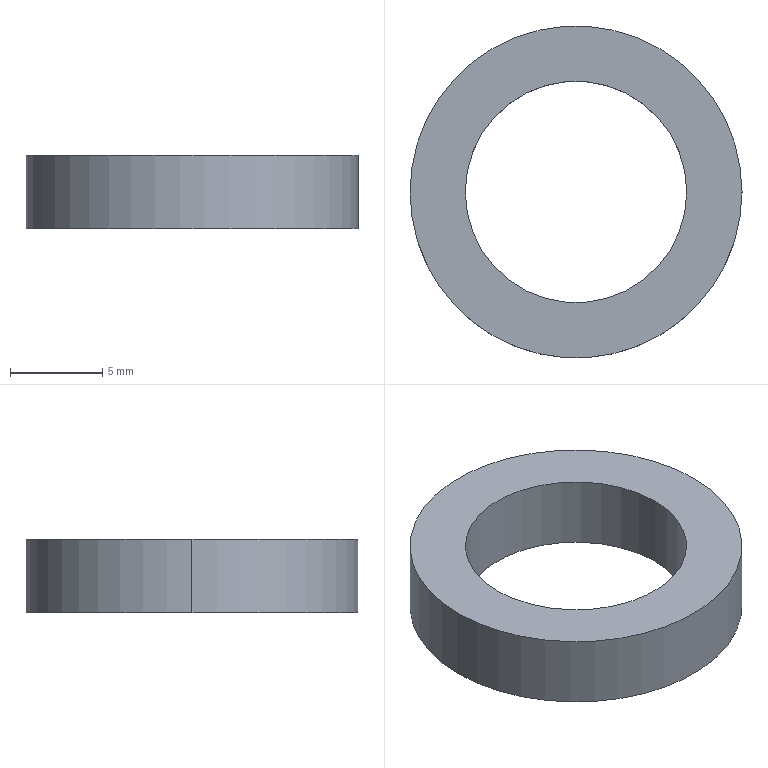Part | STEP file | 6701ZZ | 1 solid | 6 faces | box 18 x 18 x 4 mm | volume 565.487 mm3 | cylinder 4 | plane 2 | commonest cylinder face diameters 12 x2 18 x2
STEP:
#1=CARTESIAN_POINT('',(-6.,0.,4.));
#2=VERTEX_POINT('',#1);
#3=CARTESIAN_POINT('',(6.,0.,4.));
#4=VERTEX_POINT('',#3);
#5=CARTESIAN_POINT('',(0.,0.,4.));
#6=DIRECTION('',(0.,0.,1.));
#7=DIRECTION('',(1.,0.,0.));
#8=AXIS2_PLACEMENT_3D('',#5,#6,#7);
#9=CIRCLE('',#8,6.);
#10=EDGE_CURVE('',#2,#4,#9,.T.);
#11=ORIENTED_EDGE('',*,*,#10,.T.);
#12=CARTESIAN_POINT('',(6.,0.,0.));
#13=VERTEX_POINT('',#12);
#14=CARTESIAN_POINT('',(6.,0.,4.));
#15=DIRECTION('',(0.,0.,-1.));
#16=VECTOR('',#15,1000.);
#17=LINE('',#14,#16);
#18=EDGE_CURVE('',#4,#13,#17,.T.);
#19=ORIENTED_EDGE('',*,*,#18,.T.);
#20=CARTESIAN_POINT('',(-6.,0.,0.));
#21=VERTEX_POINT('',#20);
#22=CARTESIAN_POINT('',(0.,0.,0.));
#23=DIRECTION('',(0.,0.,1.));
#24=DIRECTION('',(1.,0.,0.));
#25=AXIS2_PLACEMENT_3D('',#22,#23,#24);
#26=CIRCLE('',#25,6.);
#27=EDGE_CURVE('',#21,#13,#26,.T.);
#28=ORIENTED_EDGE('',*,*,#27,.F.);
#29=CARTESIAN_POINT('',(-6.,0.,4.));
#30=DIRECTION('',(0.,0.,-1.));
#31=VECTOR('',#30,1000.);
#32=LINE('',#29,#31);
#33=EDGE_CURVE('',#2,#21,#32,.T.);
#34=ORIENTED_EDGE('',*,*,#33,.F.);
#35=EDGE_LOOP('',(#11,#19,#28,#34));
#36=FACE_OUTER_BOUND('',#35,.T.);
#37=CARTESIAN_POINT('',(0.,0.,4.));
#38=DIRECTION('',(0.,0.,-1.));
#39=DIRECTION('',(-1.,0.,0.));
#40=AXIS2_PLACEMENT_3D('',#37,#38,#39);
#41=CYLINDRICAL_SURFACE('',#40,6.);
#42=ADVANCED_FACE('',(#36),#41,.F.);
#43=CARTESIAN_POINT('',(9.,0.,4.));
#44=VERTEX_POINT('',#43);
#45=CARTESIAN_POINT('',(-9.,0.,4.));
#46=VERTEX_POINT('',#45);
#47=CARTESIAN_POINT('',(0.,0.,4.));
#48=DIRECTION('',(0.,0.,1.));
#49=DIRECTION('',(1.,0.,0.));
#50=AXIS2_PLACEMENT_3D('',#47,#48,#49);
#51=CIRCLE('',#50,9.);
#52=EDGE_CURVE('',#44,#46,#51,.T.);
#53=ORIENTED_EDGE('',*,*,#52,.F.);
#54=CARTESIAN_POINT('',(9.,0.,0.));
#55=VERTEX_POINT('',#54);
#56=CARTESIAN_POINT('',(9.,0.,4.));
#57=DIRECTION('',(0.,0.,-1.));
#58=VECTOR('',#57,1000.);
#59=LINE('',#56,#58);
#60=EDGE_CURVE('',#44,#55,#59,.T.);
#61=ORIENTED_EDGE('',*,*,#60,.T.);
#62=CARTESIAN_POINT('',(-9.,0.,0.));
#63=VERTEX_POINT('',#62);
#64=CARTESIAN_POINT('',(0.,0.,0.));
#65=DIRECTION('',(0.,0.,1.));
#66=DIRECTION('',(1.,0.,0.));
#67=AXIS2_PLACEMENT_3D('',#64,#65,#66);
#68=CIRCLE('',#67,9.);
#69=EDGE_CURVE('',#55,#63,#68,.T.);
#70=ORIENTED_EDGE('',*,*,#69,.T.);
#71=CARTESIAN_POINT('',(-9.,0.,4.));
#72=DIRECTION('',(0.,0.,-1.));
#73=VECTOR('',#72,1000.);
#74=LINE('',#71,#73);
#75=EDGE_CURVE('',#46,#63,#74,.T.);
#76=ORIENTED_EDGE('',*,*,#75,.F.);
#77=EDGE_LOOP('',(#53,#61,#70,#76));
#78=FACE_OUTER_BOUND('',#77,.T.);
#79=CARTESIAN_POINT('',(0.,0.,4.));
#80=DIRECTION('',(0.,0.,-1.));
#81=DIRECTION('',(-1.,0.,0.));
#82=AXIS2_PLACEMENT_3D('',#79,#80,#81);
#83=CYLINDRICAL_SURFACE('',#82,9.);
#84=ADVANCED_FACE('',(#78),#83,.T.);
#85=CARTESIAN_POINT('',(0.,0.,4.));
#86=DIRECTION('',(0.,0.,1.));
#87=DIRECTION('',(1.,0.,0.));
#88=AXIS2_PLACEMENT_3D('',#85,#86,#87);
#89=CIRCLE('',#88,9.);
#90=EDGE_CURVE('',#46,#44,#89,.T.);
#91=ORIENTED_EDGE('',*,*,#90,.T.);
#92=ORIENTED_EDGE('',*,*,#52,.T.);
#93=EDGE_LOOP('',(#91,#92));
#94=FACE_OUTER_BOUND('',#93,.T.);
#95=ORIENTED_EDGE('',*,*,#10,.F.);
#96=CARTESIAN_POINT('',(0.,0.,4.));
#97=DIRECTION('',(0.,0.,1.));
#98=DIRECTION('',(1.,0.,0.));
#99=AXIS2_PLACEMENT_3D('',#96,#97,#98);
#100=CIRCLE('',#99,6.);
#101=EDGE_CURVE('',#4,#2,#100,.T.);
#102=ORIENTED_EDGE('',*,*,#101,.F.);
#103=EDGE_LOOP('',(#95,#102));
#104=FACE_BOUND('',#103,.T.);
#105=CARTESIAN_POINT('',(0.,0.,4.));
#106=DIRECTION('',(0.,0.,1.));
#107=DIRECTION('',(1.,0.,0.));
#108=AXIS2_PLACEMENT_3D('',#105,#106,#107);
#109=PLANE('',#108);
#110=ADVANCED_FACE('',(#94,#104),#109,.T.);
#111=CARTESIAN_POINT('',(0.,0.,0.));
#112=DIRECTION('',(0.,0.,1.));
#113=DIRECTION('',(1.,0.,0.));
#114=AXIS2_PLACEMENT_3D('',#111,#112,#113);
#115=CIRCLE('',#114,9.);
#116=EDGE_CURVE('',#63,#55,#115,.T.);
#117=ORIENTED_EDGE('',*,*,#116,.F.);
#118=ORIENTED_EDGE('',*,*,#69,.F.);
#119=EDGE_LOOP('',(#117,#118));
#120=FACE_OUTER_BOUND('',#119,.T.);
#121=ORIENTED_EDGE('',*,*,#27,.T.);
#122=CARTESIAN_POINT('',(0.,0.,0.));
#123=DIRECTION('',(0.,0.,1.));
#124=DIRECTION('',(1.,0.,0.));
#125=AXIS2_PLACEMENT_3D('',#122,#123,#124);
#126=CIRCLE('',#125,6.);
#127=EDGE_CURVE('',#13,#21,#126,.T.);
#128=ORIENTED_EDGE('',*,*,#127,.T.);
#129=EDGE_LOOP('',(#121,#128));
#130=FACE_BOUND('',#129,.T.);
#131=CARTESIAN_POINT('',(0.,0.,0.));
#132=DIRECTION('',(0.,0.,1.));
#133=DIRECTION('',(1.,0.,0.));
#134=AXIS2_PLACEMENT_3D('',#131,#132,#133);
#135=PLANE('',#134);
#136=ADVANCED_FACE('',(#120,#130),#135,.F.);
#137=ORIENTED_EDGE('',*,*,#60,.F.);
#138=ORIENTED_EDGE('',*,*,#90,.F.);
#139=ORIENTED_EDGE('',*,*,#75,.T.);
#140=ORIENTED_EDGE('',*,*,#116,.T.);
#141=EDGE_LOOP('',(#137,#138,#139,#140));
#142=FACE_OUTER_BOUND('',#141,.T.);
#143=CARTESIAN_POINT('',(0.,0.,4.));
#144=DIRECTION('',(0.,0.,-1.));
#145=DIRECTION('',(-1.,0.,0.));
#146=AXIS2_PLACEMENT_3D('',#143,#144,#145);
#147=CYLINDRICAL_SURFACE('',#146,9.);
#148=ADVANCED_FACE('',(#142),#147,.T.);
#149=ORIENTED_EDGE('',*,*,#18,.F.);
#150=ORIENTED_EDGE('',*,*,#101,.T.);
#151=ORIENTED_EDGE('',*,*,#33,.T.);
#152=ORIENTED_EDGE('',*,*,#127,.F.);
#153=EDGE_LOOP('',(#149,#150,#151,#152));
#154=FACE_OUTER_BOUND('',#153,.T.);
#155=CARTESIAN_POINT('',(0.,0.,4.));
#156=DIRECTION('',(0.,0.,-1.));
#157=DIRECTION('',(-1.,0.,0.));
#158=AXIS2_PLACEMENT_3D('',#155,#156,#157);
#159=CYLINDRICAL_SURFACE('',#158,6.);
#160=ADVANCED_FACE('',(#154),#159,.F.);
#161=CLOSED_SHELL('',(#42,#84,#110,#136,#148,#160));
#162=MANIFOLD_SOLID_BREP('',#161);
#163=CARTESIAN_POINT('',(0.,0.,0.));
#164=DIRECTION('',(0.,0.,1.));
#165=DIRECTION('',(1.,0.,0.));
#166=AXIS2_PLACEMENT_3D('',#163,#164,#165);
#167=(LENGTH_UNIT()NAMED_UNIT(*)SI_UNIT(.MILLI.,.METRE.));
#168=UNCERTAINTY_MEASURE_WITH_UNIT(LENGTH_MEASURE(0.00001),#167,'','');
#169=(NAMED_UNIT(*)PLANE_ANGLE_UNIT()SI_UNIT($,.RADIAN.));
#170=(NAMED_UNIT(*)SI_UNIT($,.STERADIAN.)SOLID_ANGLE_UNIT());
#171=(GEOMETRIC_REPRESENTATION_CONTEXT(3)GLOBAL_UNCERTAINTY_ASSIGNED_CONTEXT((#168))GLOBAL_UNIT_ASSIGNED_CONTEXT((#167,#169,#170))REPRESENTATION_CONTEXT('',''));
#172=ADVANCED_BREP_SHAPE_REPRESENTATION('',(#162,#166),#171);